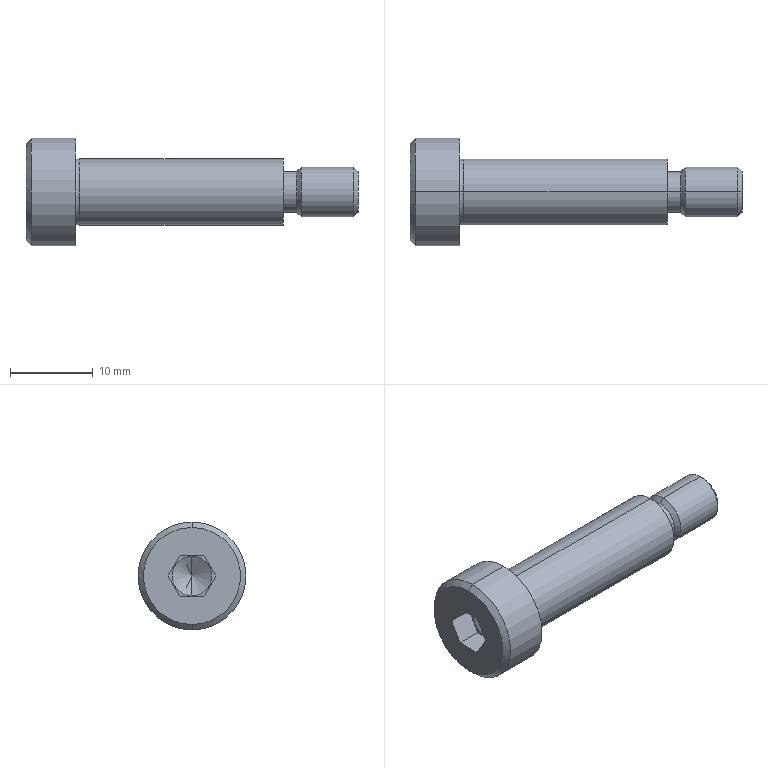Part | STEP file | MSB8-25 | 1 solid | 29 faces | box 40 x 13 x 13 mm | volume 2205 mm3 | plane 11 | cylinder 8 | cone 8 | spline 2 | commonest cylinder face diameters 4.917 x2 6 x2 8 x2 13 x2
STEP:
#1=CARTESIAN_POINT('',(0.48,0.,-4.));
#2=VERTEX_POINT('',#1);
#3=CARTESIAN_POINT('',(0.48,0.,4.));
#4=VERTEX_POINT('',#3);
#5=CARTESIAN_POINT('',(0.48,0.,0.));
#6=DIRECTION('',(1.,0.,0.));
#7=DIRECTION('',(0.,0.,-1.));
#8=AXIS2_PLACEMENT_3D('',#5,#6,#7);
#9=CIRCLE('',#8,4.);
#10=EDGE_CURVE('',#2,#4,#9,.T.);
#11=ORIENTED_EDGE('',*,*,#10,.F.);
#12=CARTESIAN_POINT('',(0.,0.,-4.));
#13=VERTEX_POINT('',#12);
#14=CARTESIAN_POINT('',(0.24,0.,-4.387));
#15=DIRECTION('',(0.,-1.,0.));
#16=DIRECTION('',(0.,0.,-1.));
#17=AXIS2_PLACEMENT_3D('',#14,#15,#16);
#18=CIRCLE('',#17,0.455);
#19=EDGE_CURVE('',#2,#13,#18,.T.);
#20=ORIENTED_EDGE('',*,*,#19,.T.);
#21=CARTESIAN_POINT('',(0.,0.,4.));
#22=VERTEX_POINT('',#21);
#23=CARTESIAN_POINT('',(0.,0.,0.));
#24=DIRECTION('',(-1.,0.,0.));
#25=DIRECTION('',(0.,0.,1.));
#26=AXIS2_PLACEMENT_3D('',#23,#24,#25);
#27=CIRCLE('',#26,4.);
#28=EDGE_CURVE('',#22,#13,#27,.T.);
#29=ORIENTED_EDGE('',*,*,#28,.F.);
#30=CARTESIAN_POINT('',(0.24,0.,4.387));
#31=DIRECTION('',(0.,1.,0.));
#32=DIRECTION('',(0.,0.,1.));
#33=AXIS2_PLACEMENT_3D('',#30,#31,#32);
#34=CIRCLE('',#33,0.455);
#35=EDGE_CURVE('',#4,#22,#34,.T.);
#36=ORIENTED_EDGE('',*,*,#35,.F.);
#37=EDGE_LOOP('',(#11,#20,#29,#36));
#38=FACE_OUTER_BOUND('',#37,.T.);
#39=CARTESIAN_POINT('',(0.48,0.,4.));
#40=CARTESIAN_POINT('',(0.48,8.,4.));
#41=CARTESIAN_POINT('',(0.48,8.,-4.));
#42=CARTESIAN_POINT('',(0.48,0.,-4.));
#43=CARTESIAN_POINT('',(0.3289,0.,3.906));
#44=CARTESIAN_POINT('',(0.3289,7.812,3.906));
#45=CARTESIAN_POINT('',(0.3289,7.812,-3.906));
#46=CARTESIAN_POINT('',(0.3289,0.,-3.906));
#47=CARTESIAN_POINT('',(0.1511,0.,3.906));
#48=CARTESIAN_POINT('',(0.1511,7.812,3.906));
#49=CARTESIAN_POINT('',(0.1511,7.812,-3.906));
#50=CARTESIAN_POINT('',(0.1511,0.,-3.906));
#51=CARTESIAN_POINT('',(0.,0.,4.));
#52=CARTESIAN_POINT('',(0.,8.,4.));
#53=CARTESIAN_POINT('',(0.,8.,-4.));
#54=CARTESIAN_POINT('',(0.,0.,-4.));
#55=(BOUNDED_SURFACE()B_SPLINE_SURFACE(3,3,((#39,#40,#41,#42),(#43,#44,#45,#46),(#47,#48,#49,#50),(#51,#52,#53,#54)),.UNSPECIFIED.,.F.,.F.,.F.)B_SPLINE_SURFACE_WITH_KNOTS((4,4),(4,4),(0.,1.),(0.,1.),.UNSPECIFIED.)GEOMETRIC_REPRESENTATION_ITEM()RATIONAL_B_SPLINE_SURFACE(((1.,0.3333,0.3333,1.),(0.8997,0.2999,0.2999,0.8997),(0.8997,0.2999,0.2999,0.8997),(1.,0.3333,0.3333,1.)))REPRESENTATION_ITEM('')SURFACE());
#56=ADVANCED_FACE('',(#38),#55,.F.);
#57=ORIENTED_EDGE('',*,*,#10,.T.);
#58=CARTESIAN_POINT('',(25.,0.,4.));
#59=VERTEX_POINT('',#58);
#60=CARTESIAN_POINT('',(12.74,0.,4.));
#61=DIRECTION('',(1.,0.,0.));
#62=VECTOR('',#61,1000.);
#63=LINE('',#60,#62);
#64=EDGE_CURVE('',#4,#59,#63,.T.);
#65=ORIENTED_EDGE('',*,*,#64,.T.);
#66=CARTESIAN_POINT('',(25.,0.,-4.));
#67=VERTEX_POINT('',#66);
#68=CARTESIAN_POINT('',(25.,0.,0.));
#69=DIRECTION('',(-1.,0.,0.));
#70=DIRECTION('',(0.,0.,-1.));
#71=AXIS2_PLACEMENT_3D('',#68,#69,#70);
#72=CIRCLE('',#71,4.);
#73=EDGE_CURVE('',#59,#67,#72,.T.);
#74=ORIENTED_EDGE('',*,*,#73,.T.);
#75=CARTESIAN_POINT('',(12.74,0.,-4.));
#76=DIRECTION('',(1.,0.,0.));
#77=VECTOR('',#76,1000.);
#78=LINE('',#75,#77);
#79=EDGE_CURVE('',#2,#67,#78,.T.);
#80=ORIENTED_EDGE('',*,*,#79,.F.);
#81=EDGE_LOOP('',(#57,#65,#74,#80));
#82=FACE_OUTER_BOUND('',#81,.T.);
#83=CARTESIAN_POINT('',(12.74,0.,0.));
#84=DIRECTION('',(1.,0.,0.));
#85=DIRECTION('',(0.,0.,-1.));
#86=AXIS2_PLACEMENT_3D('',#83,#84,#85);
#87=CYLINDRICAL_SURFACE('',#86,4.);
#88=ADVANCED_FACE('',(#82),#87,.T.);
#89=CARTESIAN_POINT('',(25.,0.,2.459));
#90=VERTEX_POINT('',#89);
#91=CARTESIAN_POINT('',(25.,0.,-2.459));
#92=VERTEX_POINT('',#91);
#93=CARTESIAN_POINT('',(25.,0.,0.));
#94=DIRECTION('',(-1.,0.,0.));
#95=DIRECTION('',(0.,0.,-1.));
#96=AXIS2_PLACEMENT_3D('',#93,#94,#95);
#97=CIRCLE('',#96,2.459);
#98=EDGE_CURVE('',#90,#92,#97,.T.);
#99=ORIENTED_EDGE('',*,*,#98,.F.);
#100=CARTESIAN_POINT('',(26.617,0.,2.459));
#101=VERTEX_POINT('',#100);
#102=CARTESIAN_POINT('',(25.809,0.,2.459));
#103=DIRECTION('',(1.,0.,0.));
#104=VECTOR('',#103,1000.);
#105=LINE('',#102,#104);
#106=EDGE_CURVE('',#90,#101,#105,.T.);
#107=ORIENTED_EDGE('',*,*,#106,.T.);
#108=CARTESIAN_POINT('',(26.617,0.,-2.459));
#109=VERTEX_POINT('',#108);
#110=CARTESIAN_POINT('',(26.617,0.,0.));
#111=DIRECTION('',(-1.,0.,0.));
#112=DIRECTION('',(0.,0.,-1.));
#113=AXIS2_PLACEMENT_3D('',#110,#111,#112);
#114=CIRCLE('',#113,2.459);
#115=EDGE_CURVE('',#101,#109,#114,.T.);
#116=ORIENTED_EDGE('',*,*,#115,.T.);
#117=CARTESIAN_POINT('',(25.809,0.,-2.459));
#118=DIRECTION('',(1.,0.,0.));
#119=VECTOR('',#118,1000.);
#120=LINE('',#117,#119);
#121=EDGE_CURVE('',#92,#109,#120,.T.);
#122=ORIENTED_EDGE('',*,*,#121,.F.);
#123=EDGE_LOOP('',(#99,#107,#116,#122));
#124=FACE_OUTER_BOUND('',#123,.T.);
#125=CARTESIAN_POINT('',(25.809,0.,0.));
#126=DIRECTION('',(1.,0.,0.));
#127=DIRECTION('',(0.,0.,-1.));
#128=AXIS2_PLACEMENT_3D('',#125,#126,#127);
#129=CYLINDRICAL_SURFACE('',#128,2.459);
#130=ADVANCED_FACE('',(#124),#129,.T.);
#131=ORIENTED_EDGE('',*,*,#115,.F.);
#132=CARTESIAN_POINT('',(27.158,0.,3.));
#133=VERTEX_POINT('',#132);
#134=CARTESIAN_POINT('',(27.158,0.,3.));
#135=DIRECTION('',(0.7071,0.,0.7071));
#136=VECTOR('',#135,1000.);
#137=LINE('',#134,#136);
#138=EDGE_CURVE('',#101,#133,#137,.T.);
#139=ORIENTED_EDGE('',*,*,#138,.T.);
#140=CARTESIAN_POINT('',(27.158,0.,-3.));
#141=VERTEX_POINT('',#140);
#142=CARTESIAN_POINT('',(27.158,0.,0.));
#143=DIRECTION('',(-1.,0.,0.));
#144=DIRECTION('',(0.,1.,0.));
#145=AXIS2_PLACEMENT_3D('',#142,#143,#144);
#146=CIRCLE('',#145,3.);
#147=EDGE_CURVE('',#133,#141,#146,.T.);
#148=ORIENTED_EDGE('',*,*,#147,.T.);
#149=CARTESIAN_POINT('',(27.158,0.,-3.));
#150=DIRECTION('',(0.7071,0.,-0.7071));
#151=VECTOR('',#150,1000.);
#152=LINE('',#149,#151);
#153=EDGE_CURVE('',#109,#141,#152,.T.);
#154=ORIENTED_EDGE('',*,*,#153,.F.);
#155=EDGE_LOOP('',(#131,#139,#148,#154));
#156=FACE_OUTER_BOUND('',#155,.T.);
#157=CARTESIAN_POINT('',(27.158,0.,0.));
#158=DIRECTION('',(1.,0.,0.));
#159=DIRECTION('',(0.,0.,-1.));
#160=AXIS2_PLACEMENT_3D('',#157,#158,#159);
#161=CONICAL_SURFACE('',#160,3.,0.7854);
#162=ADVANCED_FACE('',(#156),#161,.T.);
#163=CARTESIAN_POINT('',(-5.35,0.,-6.5));
#164=VERTEX_POINT('',#163);
#165=CARTESIAN_POINT('',(-5.35,0.,6.5));
#166=VERTEX_POINT('',#165);
#167=CARTESIAN_POINT('',(-5.35,0.,0.));
#168=DIRECTION('',(1.,0.,0.));
#169=DIRECTION('',(0.,0.,-1.));
#170=AXIS2_PLACEMENT_3D('',#167,#168,#169);
#171=CIRCLE('',#170,6.5);
#172=EDGE_CURVE('',#164,#166,#171,.T.);
#173=ORIENTED_EDGE('',*,*,#172,.T.);
#174=CARTESIAN_POINT('',(0.,0.,6.5));
#175=VERTEX_POINT('',#174);
#176=CARTESIAN_POINT('',(-2.675,0.,6.5));
#177=DIRECTION('',(1.,0.,0.));
#178=VECTOR('',#177,1000.);
#179=LINE('',#176,#178);
#180=EDGE_CURVE('',#166,#175,#179,.T.);
#181=ORIENTED_EDGE('',*,*,#180,.T.);
#182=CARTESIAN_POINT('',(0.,0.,-6.5));
#183=VERTEX_POINT('',#182);
#184=CARTESIAN_POINT('',(0.,0.,0.));
#185=DIRECTION('',(1.,0.,0.));
#186=DIRECTION('',(0.,0.,-1.));
#187=AXIS2_PLACEMENT_3D('',#184,#185,#186);
#188=CIRCLE('',#187,6.5);
#189=EDGE_CURVE('',#183,#175,#188,.T.);
#190=ORIENTED_EDGE('',*,*,#189,.F.);
#191=CARTESIAN_POINT('',(-2.675,0.,-6.5));
#192=DIRECTION('',(1.,0.,0.));
#193=VECTOR('',#192,1000.);
#194=LINE('',#191,#193);
#195=EDGE_CURVE('',#164,#183,#194,.T.);
#196=ORIENTED_EDGE('',*,*,#195,.F.);
#197=EDGE_LOOP('',(#173,#181,#190,#196));
#198=FACE_OUTER_BOUND('',#197,.T.);
#199=CARTESIAN_POINT('',(-2.675,0.,0.));
#200=DIRECTION('',(1.,0.,0.));
#201=DIRECTION('',(0.,0.,-1.));
#202=AXIS2_PLACEMENT_3D('',#199,#200,#201);
#203=CYLINDRICAL_SURFACE('',#202,6.5);
#204=ADVANCED_FACE('',(#198),#203,.T.);
#205=ORIENTED_EDGE('',*,*,#147,.F.);
#206=CARTESIAN_POINT('',(33.459,0.,3.));
#207=VERTEX_POINT('',#206);
#208=CARTESIAN_POINT('',(30.308,0.,3.));
#209=DIRECTION('',(1.,0.,0.));
#210=VECTOR('',#209,1000.);
#211=LINE('',#208,#210);
#212=EDGE_CURVE('',#133,#207,#211,.T.);
#213=ORIENTED_EDGE('',*,*,#212,.T.);
#214=CARTESIAN_POINT('',(33.459,0.,-3.));
#215=VERTEX_POINT('',#214);
#216=CARTESIAN_POINT('',(33.459,0.,0.));
#217=DIRECTION('',(-1.,0.,0.));
#218=DIRECTION('',(0.,0.,-1.));
#219=AXIS2_PLACEMENT_3D('',#216,#217,#218);
#220=CIRCLE('',#219,3.);
#221=EDGE_CURVE('',#207,#215,#220,.T.);
#222=ORIENTED_EDGE('',*,*,#221,.T.);
#223=CARTESIAN_POINT('',(30.308,0.,-3.));
#224=DIRECTION('',(1.,0.,0.));
#225=VECTOR('',#224,1000.);
#226=LINE('',#223,#225);
#227=EDGE_CURVE('',#141,#215,#226,.T.);
#228=ORIENTED_EDGE('',*,*,#227,.F.);
#229=EDGE_LOOP('',(#205,#213,#222,#228));
#230=FACE_OUTER_BOUND('',#229,.T.);
#231=CARTESIAN_POINT('',(30.308,0.,0.));
#232=DIRECTION('',(1.,0.,0.));
#233=DIRECTION('',(0.,0.,-1.));
#234=AXIS2_PLACEMENT_3D('',#231,#232,#233);
#235=CYLINDRICAL_SURFACE('',#234,3.);
#236=ADVANCED_FACE('',(#230),#235,.T.);
#237=CARTESIAN_POINT('',(-6.,0.,-5.85));
#238=VERTEX_POINT('',#237);
#239=CARTESIAN_POINT('',(-6.,0.,5.85));
#240=VERTEX_POINT('',#239);
#241=CARTESIAN_POINT('',(-6.,0.,0.));
#242=DIRECTION('',(1.,0.,0.));
#243=DIRECTION('',(0.,0.,-1.));
#244=AXIS2_PLACEMENT_3D('',#241,#242,#243);
#245=CIRCLE('',#244,5.85);
#246=EDGE_CURVE('',#238,#240,#245,.T.);
#247=ORIENTED_EDGE('',*,*,#246,.T.);
#248=CARTESIAN_POINT('',(-5.35,0.,6.5));
#249=DIRECTION('',(0.7071,0.,0.7071));
#250=VECTOR('',#249,1000.);
#251=LINE('',#248,#250);
#252=EDGE_CURVE('',#240,#166,#251,.T.);
#253=ORIENTED_EDGE('',*,*,#252,.T.);
#254=ORIENTED_EDGE('',*,*,#172,.F.);
#255=CARTESIAN_POINT('',(-5.35,0.,-6.5));
#256=DIRECTION('',(0.7071,0.,-0.7071));
#257=VECTOR('',#256,1000.);
#258=LINE('',#255,#257);
#259=EDGE_CURVE('',#238,#164,#258,.T.);
#260=ORIENTED_EDGE('',*,*,#259,.F.);
#261=EDGE_LOOP('',(#247,#253,#254,#260));
#262=FACE_OUTER_BOUND('',#261,.T.);
#263=CARTESIAN_POINT('',(-5.35,0.,0.));
#264=DIRECTION('',(1.,0.,0.));
#265=DIRECTION('',(0.,0.,-1.));
#266=AXIS2_PLACEMENT_3D('',#263,#264,#265);
#267=CONICAL_SURFACE('',#266,6.5,0.7854);
#268=ADVANCED_FACE('',(#262),#267,.T.);
#269=CARTESIAN_POINT('',(34.,0.,2.459));
#270=VERTEX_POINT('',#269);
#271=CARTESIAN_POINT('',(34.,0.,-2.459));
#272=VERTEX_POINT('',#271);
#273=CARTESIAN_POINT('',(34.,0.,0.));
#274=DIRECTION('',(-1.,0.,0.));
#275=DIRECTION('',(0.,0.,1.));
#276=AXIS2_PLACEMENT_3D('',#273,#274,#275);
#277=CIRCLE('',#276,2.459);
#278=EDGE_CURVE('',#270,#272,#277,.T.);
#279=ORIENTED_EDGE('',*,*,#278,.T.);
#280=CARTESIAN_POINT('',(33.459,0.,-3.));
#281=DIRECTION('',(-0.7071,0.,-0.7071));
#282=VECTOR('',#281,1000.);
#283=LINE('',#280,#282);
#284=EDGE_CURVE('',#272,#215,#283,.T.);
#285=ORIENTED_EDGE('',*,*,#284,.T.);
#286=ORIENTED_EDGE('',*,*,#221,.F.);
#287=CARTESIAN_POINT('',(33.459,0.,3.));
#288=DIRECTION('',(-0.7071,0.,0.7071));
#289=VECTOR('',#288,1000.);
#290=LINE('',#287,#289);
#291=EDGE_CURVE('',#270,#207,#290,.T.);
#292=ORIENTED_EDGE('',*,*,#291,.F.);
#293=EDGE_LOOP('',(#279,#285,#286,#292));
#294=FACE_OUTER_BOUND('',#293,.T.);
#295=CARTESIAN_POINT('',(33.459,0.,0.));
#296=DIRECTION('',(-1.,0.,0.));
#297=DIRECTION('',(0.,0.,1.));
#298=AXIS2_PLACEMENT_3D('',#295,#296,#297);
#299=CONICAL_SURFACE('',#298,3.,0.7854);
#300=ADVANCED_FACE('',(#294),#299,.T.);
#301=CARTESIAN_POINT('',(-1.614,0.,0.));
#302=VERTEX_POINT('',#301);
#303=CARTESIAN_POINT('',(-3.,0.,2.4));
#304=VERTEX_POINT('',#303);
#305=CARTESIAN_POINT('',(-3.,0.,2.4));
#306=DIRECTION('',(-0.5,0.,0.866));
#307=VECTOR('',#306,1000.);
#308=LINE('',#305,#307);
#309=EDGE_CURVE('',#302,#304,#308,.T.);
#310=ORIENTED_EDGE('',*,*,#309,.F.);
#311=CARTESIAN_POINT('',(-3.,0.,-2.4));
#312=VERTEX_POINT('',#311);
#313=CARTESIAN_POINT('',(-3.,0.,-2.4));
#314=DIRECTION('',(-0.5,0.,-0.866));
#315=VECTOR('',#314,1000.);
#316=LINE('',#313,#315);
#317=EDGE_CURVE('',#302,#312,#316,.T.);
#318=ORIENTED_EDGE('',*,*,#317,.T.);
#319=CARTESIAN_POINT('',(-3.,0.,0.));
#320=DIRECTION('',(-1.,0.,0.));
#321=DIRECTION('',(0.,0.,1.));
#322=AXIS2_PLACEMENT_3D('',#319,#320,#321);
#323=CIRCLE('',#322,2.4);
#324=EDGE_CURVE('',#312,#304,#323,.T.);
#325=ORIENTED_EDGE('',*,*,#324,.T.);
#326=EDGE_LOOP('',(#310,#318,#325));
#327=FACE_OUTER_BOUND('',#326,.T.);
#328=CARTESIAN_POINT('',(-3.,0.,0.));
#329=DIRECTION('',(-1.,0.,0.));
#330=DIRECTION('',(0.,0.,1.));
#331=AXIS2_PLACEMENT_3D('',#328,#329,#330);
#332=CONICAL_SURFACE('',#331,2.4,1.047);
#333=ADVANCED_FACE('',(#327),#332,.F.);
#334=ORIENTED_EDGE('',*,*,#64,.F.);
#335=CARTESIAN_POINT('',(0.48,0.,0.));
#336=DIRECTION('',(1.,0.,0.));
#337=DIRECTION('',(0.,0.,-1.));
#338=AXIS2_PLACEMENT_3D('',#335,#336,#337);
#339=CIRCLE('',#338,4.);
#340=EDGE_CURVE('',#4,#2,#339,.T.);
#341=ORIENTED_EDGE('',*,*,#340,.T.);
#342=ORIENTED_EDGE('',*,*,#79,.T.);
#343=CARTESIAN_POINT('',(25.,0.,0.));
#344=DIRECTION('',(-1.,0.,0.));
#345=DIRECTION('',(0.,0.,-1.));
#346=AXIS2_PLACEMENT_3D('',#343,#344,#345);
#347=CIRCLE('',#346,4.);
#348=EDGE_CURVE('',#67,#59,#347,.T.);
#349=ORIENTED_EDGE('',*,*,#348,.T.);
#350=EDGE_LOOP('',(#334,#341,#342,#349));
#351=FACE_OUTER_BOUND('',#350,.T.);
#352=CARTESIAN_POINT('',(12.74,0.,0.));
#353=DIRECTION('',(1.,0.,0.));
#354=DIRECTION('',(0.,0.,-1.));
#355=AXIS2_PLACEMENT_3D('',#352,#353,#354);
#356=CYLINDRICAL_SURFACE('',#355,4.);
#357=ADVANCED_FACE('',(#351),#356,.T.);
#358=ORIENTED_EDGE('',*,*,#19,.F.);
#359=ORIENTED_EDGE('',*,*,#340,.F.);
#360=ORIENTED_EDGE('',*,*,#35,.T.);
#361=CARTESIAN_POINT('',(0.,0.,0.));
#362=DIRECTION('',(-1.,0.,0.));
#363=DIRECTION('',(0.,0.,1.));
#364=AXIS2_PLACEMENT_3D('',#361,#362,#363);
#365=CIRCLE('',#364,4.);
#366=EDGE_CURVE('',#13,#22,#365,.T.);
#367=ORIENTED_EDGE('',*,*,#366,.F.);
#368=EDGE_LOOP('',(#358,#359,#360,#367));
#369=FACE_OUTER_BOUND('',#368,.T.);
#370=CARTESIAN_POINT('',(0.48,0.,-4.));
#371=CARTESIAN_POINT('',(0.48,-8.,-4.));
#372=CARTESIAN_POINT('',(0.48,-8.,4.));
#373=CARTESIAN_POINT('',(0.48,0.,4.));
#374=CARTESIAN_POINT('',(0.3289,0.,-3.906));
#375=CARTESIAN_POINT('',(0.3289,-7.812,-3.906));
#376=CARTESIAN_POINT('',(0.3289,-7.812,3.906));
#377=CARTESIAN_POINT('',(0.3289,0.,3.906));
#378=CARTESIAN_POINT('',(0.1511,0.,-3.906));
#379=CARTESIAN_POINT('',(0.1511,-7.812,-3.906));
#380=CARTESIAN_POINT('',(0.1511,-7.812,3.906));
#381=CARTESIAN_POINT('',(0.1511,0.,3.906));
#382=CARTESIAN_POINT('',(0.,0.,-4.));
#383=CARTESIAN_POINT('',(0.,-8.,-4.));
#384=CARTESIAN_POINT('',(0.,-8.,4.));
#385=CARTESIAN_POINT('',(0.,0.,4.));
#386=(BOUNDED_SURFACE()B_SPLINE_SURFACE(3,3,((#370,#371,#372,#373),(#374,#375,#376,#377),(#378,#379,#380,#381),(#382,#383,#384,#385)),.UNSPECIFIED.,.F.,.F.,.F.)B_SPLINE_SURFACE_WITH_KNOTS((4,4),(4,4),(0.,1.),(0.,1.),.UNSPECIFIED.)GEOMETRIC_REPRESENTATION_ITEM()RATIONAL_B_SPLINE_SURFACE(((1.,0.3333,0.3333,1.),(0.8997,0.2999,0.2999,0.8997),(0.8997,0.2999,0.2999,0.8997),(1.,0.3333,0.3333,1.)))REPRESENTATION_ITEM('')SURFACE());
#387=ADVANCED_FACE('',(#369),#386,.F.);
#388=CARTESIAN_POINT('',(25.,0.,0.));
#389=DIRECTION('',(-1.,0.,0.));
#390=DIRECTION('',(0.,0.,-1.));
#391=AXIS2_PLACEMENT_3D('',#388,#389,#390);
#392=CIRCLE('',#391,2.459);
#393=EDGE_CURVE('',#92,#90,#392,.T.);
#394=ORIENTED_EDGE('',*,*,#393,.T.);
#395=ORIENTED_EDGE('',*,*,#98,.T.);
#396=EDGE_LOOP('',(#394,#395));
#397=FACE_BOUND('',#396,.T.);
#398=ORIENTED_EDGE('',*,*,#348,.F.);
#399=ORIENTED_EDGE('',*,*,#73,.F.);
#400=EDGE_LOOP('',(#398,#399));
#401=FACE_OUTER_BOUND('',#400,.T.);
#402=CARTESIAN_POINT('',(25.,3.229,0.));
#403=DIRECTION('',(1.,0.,0.));
#404=DIRECTION('',(0.,0.,-1.));
#405=AXIS2_PLACEMENT_3D('',#402,#403,#404);
#406=PLANE('',#405);
#407=ADVANCED_FACE('',(#397,#401),#406,.T.);
#408=ORIENTED_EDGE('',*,*,#106,.F.);
#409=ORIENTED_EDGE('',*,*,#393,.F.);
#410=ORIENTED_EDGE('',*,*,#121,.T.);
#411=CARTESIAN_POINT('',(26.617,0.,0.));
#412=DIRECTION('',(-1.,0.,0.));
#413=DIRECTION('',(0.,0.,-1.));
#414=AXIS2_PLACEMENT_3D('',#411,#412,#413);
#415=CIRCLE('',#414,2.459);
#416=EDGE_CURVE('',#109,#101,#415,.T.);
#417=ORIENTED_EDGE('',*,*,#416,.T.);
#418=EDGE_LOOP('',(#408,#409,#410,#417));
#419=FACE_OUTER_BOUND('',#418,.T.);
#420=CARTESIAN_POINT('',(25.809,0.,0.));
#421=DIRECTION('',(1.,0.,0.));
#422=DIRECTION('',(0.,0.,-1.));
#423=AXIS2_PLACEMENT_3D('',#420,#421,#422);
#424=CYLINDRICAL_SURFACE('',#423,2.459);
#425=ADVANCED_FACE('',(#419),#424,.T.);
#426=ORIENTED_EDGE('',*,*,#28,.T.);
#427=ORIENTED_EDGE('',*,*,#366,.T.);
#428=EDGE_LOOP('',(#426,#427));
#429=FACE_BOUND('',#428,.T.);
#430=ORIENTED_EDGE('',*,*,#189,.T.);
#431=CARTESIAN_POINT('',(0.,0.,0.));
#432=DIRECTION('',(1.,0.,0.));
#433=DIRECTION('',(0.,0.,-1.));
#434=AXIS2_PLACEMENT_3D('',#431,#432,#433);
#435=CIRCLE('',#434,6.5);
#436=EDGE_CURVE('',#175,#183,#435,.T.);
#437=ORIENTED_EDGE('',*,*,#436,.T.);
#438=EDGE_LOOP('',(#430,#437));
#439=FACE_OUTER_BOUND('',#438,.T.);
#440=CARTESIAN_POINT('',(0.,5.25,0.));
#441=DIRECTION('',(1.,0.,0.));
#442=DIRECTION('',(0.,0.,-1.));
#443=AXIS2_PLACEMENT_3D('',#440,#441,#442);
#444=PLANE('',#443);
#445=ADVANCED_FACE('',(#429,#439),#444,.T.);
#446=ORIENTED_EDGE('',*,*,#138,.F.);
#447=ORIENTED_EDGE('',*,*,#416,.F.);
#448=ORIENTED_EDGE('',*,*,#153,.T.);
#449=CARTESIAN_POINT('',(27.158,0.,0.));
#450=DIRECTION('',(-1.,0.,0.));
#451=DIRECTION('',(0.,1.,0.));
#452=AXIS2_PLACEMENT_3D('',#449,#450,#451);
#453=CIRCLE('',#452,3.);
#454=EDGE_CURVE('',#141,#133,#453,.T.);
#455=ORIENTED_EDGE('',*,*,#454,.T.);
#456=EDGE_LOOP('',(#446,#447,#448,#455));
#457=FACE_OUTER_BOUND('',#456,.T.);
#458=CARTESIAN_POINT('',(27.158,0.,0.));
#459=DIRECTION('',(1.,0.,0.));
#460=DIRECTION('',(0.,0.,-1.));
#461=AXIS2_PLACEMENT_3D('',#458,#459,#460);
#462=CONICAL_SURFACE('',#461,3.,0.7854);
#463=ADVANCED_FACE('',(#457),#462,.T.);
#464=ORIENTED_EDGE('',*,*,#180,.F.);
#465=CARTESIAN_POINT('',(-5.35,0.,0.));
#466=DIRECTION('',(1.,0.,0.));
#467=DIRECTION('',(0.,0.,-1.));
#468=AXIS2_PLACEMENT_3D('',#465,#466,#467);
#469=CIRCLE('',#468,6.5);
#470=EDGE_CURVE('',#166,#164,#469,.T.);
#471=ORIENTED_EDGE('',*,*,#470,.T.);
#472=ORIENTED_EDGE('',*,*,#195,.T.);
#473=ORIENTED_EDGE('',*,*,#436,.F.);
#474=EDGE_LOOP('',(#464,#471,#472,#473));
#475=FACE_OUTER_BOUND('',#474,.T.);
#476=CARTESIAN_POINT('',(-2.675,0.,0.));
#477=DIRECTION('',(1.,0.,0.));
#478=DIRECTION('',(0.,0.,-1.));
#479=AXIS2_PLACEMENT_3D('',#476,#477,#478);
#480=CYLINDRICAL_SURFACE('',#479,6.5);
#481=ADVANCED_FACE('',(#475),#480,.T.);
#482=ORIENTED_EDGE('',*,*,#212,.F.);
#483=ORIENTED_EDGE('',*,*,#454,.F.);
#484=ORIENTED_EDGE('',*,*,#227,.T.);
#485=CARTESIAN_POINT('',(33.459,0.,0.));
#486=DIRECTION('',(-1.,0.,0.));
#487=DIRECTION('',(0.,0.,-1.));
#488=AXIS2_PLACEMENT_3D('',#485,#486,#487);
#489=CIRCLE('',#488,3.);
#490=EDGE_CURVE('',#215,#207,#489,.T.);
#491=ORIENTED_EDGE('',*,*,#490,.T.);
#492=EDGE_LOOP('',(#482,#483,#484,#491));
#493=FACE_OUTER_BOUND('',#492,.T.);
#494=CARTESIAN_POINT('',(30.308,0.,0.));
#495=DIRECTION('',(1.,0.,0.));
#496=DIRECTION('',(0.,0.,-1.));
#497=AXIS2_PLACEMENT_3D('',#494,#495,#496);
#498=CYLINDRICAL_SURFACE('',#497,3.);
#499=ADVANCED_FACE('',(#493),#498,.T.);
#500=ORIENTED_EDGE('',*,*,#252,.F.);
#501=CARTESIAN_POINT('',(-6.,0.,0.));
#502=DIRECTION('',(1.,0.,0.));
#503=DIRECTION('',(0.,0.,-1.));
#504=AXIS2_PLACEMENT_3D('',#501,#502,#503);
#505=CIRCLE('',#504,5.85);
#506=EDGE_CURVE('',#240,#238,#505,.T.);
#507=ORIENTED_EDGE('',*,*,#506,.T.);
#508=ORIENTED_EDGE('',*,*,#259,.T.);
#509=ORIENTED_EDGE('',*,*,#470,.F.);
#510=EDGE_LOOP('',(#500,#507,#508,#509));
#511=FACE_OUTER_BOUND('',#510,.T.);
#512=CARTESIAN_POINT('',(-5.35,0.,0.));
#513=DIRECTION('',(1.,0.,0.));
#514=DIRECTION('',(0.,0.,-1.));
#515=AXIS2_PLACEMENT_3D('',#512,#513,#514);
#516=CONICAL_SURFACE('',#515,6.5,0.7854);
#517=ADVANCED_FACE('',(#511),#516,.T.);
#518=ORIENTED_EDGE('',*,*,#284,.F.);
#519=CARTESIAN_POINT('',(34.,0.,0.));
#520=DIRECTION('',(-1.,0.,0.));
#521=DIRECTION('',(0.,0.,1.));
#522=AXIS2_PLACEMENT_3D('',#519,#520,#521);
#523=CIRCLE('',#522,2.459);
#524=EDGE_CURVE('',#272,#270,#523,.T.);
#525=ORIENTED_EDGE('',*,*,#524,.T.);
#526=ORIENTED_EDGE('',*,*,#291,.T.);
#527=ORIENTED_EDGE('',*,*,#490,.F.);
#528=EDGE_LOOP('',(#518,#525,#526,#527));
#529=FACE_OUTER_BOUND('',#528,.T.);
#530=CARTESIAN_POINT('',(33.459,0.,0.));
#531=DIRECTION('',(-1.,0.,0.));
#532=DIRECTION('',(0.,0.,1.));
#533=AXIS2_PLACEMENT_3D('',#530,#531,#532);
#534=CONICAL_SURFACE('',#533,3.,0.7854);
#535=ADVANCED_FACE('',(#529),#534,.T.);
#536=ORIENTED_EDGE('',*,*,#246,.F.);
#537=ORIENTED_EDGE('',*,*,#506,.F.);
#538=EDGE_LOOP('',(#536,#537));
#539=FACE_OUTER_BOUND('',#538,.T.);
#540=CARTESIAN_POINT('',(-6.,-1.443,-2.5));
#541=VERTEX_POINT('',#540);
#542=CARTESIAN_POINT('',(-6.,1.443,-2.5));
#543=VERTEX_POINT('',#542);
#544=CARTESIAN_POINT('',(-6.,4.125,-2.5));
#545=DIRECTION('',(0.,1.,0.));
#546=VECTOR('',#545,1000.);
#547=LINE('',#544,#546);
#548=EDGE_CURVE('',#541,#543,#547,.T.);
#549=ORIENTED_EDGE('',*,*,#548,.T.);
#550=CARTESIAN_POINT('',(-6.,2.887,0.));
#551=VERTEX_POINT('',#550);
#552=CARTESIAN_POINT('',(-6.,1.443,-2.5));
#553=DIRECTION('',(0.,0.5,0.866));
#554=VECTOR('',#553,1000.);
#555=LINE('',#552,#554);
#556=EDGE_CURVE('',#543,#551,#555,.T.);
#557=ORIENTED_EDGE('',*,*,#556,.T.);
#558=CARTESIAN_POINT('',(-6.,1.443,2.5));
#559=VERTEX_POINT('',#558);
#560=CARTESIAN_POINT('',(-6.,2.887,0.));
#561=DIRECTION('',(0.,-0.5,0.866));
#562=VECTOR('',#561,1000.);
#563=LINE('',#560,#562);
#564=EDGE_CURVE('',#551,#559,#563,.T.);
#565=ORIENTED_EDGE('',*,*,#564,.T.);
#566=CARTESIAN_POINT('',(-6.,-1.443,2.5));
#567=VERTEX_POINT('',#566);
#568=CARTESIAN_POINT('',(-6.,4.125,2.5));
#569=DIRECTION('',(0.,-1.,0.));
#570=VECTOR('',#569,1000.);
#571=LINE('',#568,#570);
#572=EDGE_CURVE('',#559,#567,#571,.T.);
#573=ORIENTED_EDGE('',*,*,#572,.T.);
#574=CARTESIAN_POINT('',(-6.,-2.887,0.));
#575=VERTEX_POINT('',#574);
#576=CARTESIAN_POINT('',(-6.,-1.443,2.5));
#577=DIRECTION('',(0.,-0.5,-0.866));
#578=VECTOR('',#577,1000.);
#579=LINE('',#576,#578);
#580=EDGE_CURVE('',#567,#575,#579,.T.);
#581=ORIENTED_EDGE('',*,*,#580,.T.);
#582=CARTESIAN_POINT('',(-6.,-2.887,0.));
#583=DIRECTION('',(0.,0.5,-0.866));
#584=VECTOR('',#583,1000.);
#585=LINE('',#582,#584);
#586=EDGE_CURVE('',#575,#541,#585,.T.);
#587=ORIENTED_EDGE('',*,*,#586,.T.);
#588=EDGE_LOOP('',(#549,#557,#565,#573,#581,#587));
#589=FACE_BOUND('',#588,.T.);
#590=CARTESIAN_POINT('',(-6.,4.125,0.));
#591=DIRECTION('',(-1.,0.,0.));
#592=DIRECTION('',(0.,0.,1.));
#593=AXIS2_PLACEMENT_3D('',#590,#591,#592);
#594=PLANE('',#593);
#595=ADVANCED_FACE('',(#539,#589),#594,.T.);
#596=ORIENTED_EDGE('',*,*,#278,.F.);
#597=ORIENTED_EDGE('',*,*,#524,.F.);
#598=EDGE_LOOP('',(#596,#597));
#599=FACE_OUTER_BOUND('',#598,.T.);
#600=CARTESIAN_POINT('',(34.,1.229,0.));
#601=DIRECTION('',(1.,0.,0.));
#602=DIRECTION('',(0.,0.,-1.));
#603=AXIS2_PLACEMENT_3D('',#600,#601,#602);
#604=PLANE('',#603);
#605=ADVANCED_FACE('',(#599),#604,.T.);
#606=CARTESIAN_POINT('',(-3.,2.887,0.));
#607=VERTEX_POINT('',#606);
#608=CARTESIAN_POINT('',(-6.,2.887,0.));
#609=DIRECTION('',(1.,0.,0.));
#610=VECTOR('',#609,1000.);
#611=LINE('',#608,#610);
#612=EDGE_CURVE('',#551,#607,#611,.T.);
#613=ORIENTED_EDGE('',*,*,#612,.F.);
#614=ORIENTED_EDGE('',*,*,#556,.F.);
#615=CARTESIAN_POINT('',(-3.,1.443,-2.5));
#616=VERTEX_POINT('',#615);
#617=CARTESIAN_POINT('',(-6.,1.443,-2.5));
#618=DIRECTION('',(-1.,0.,0.));
#619=VECTOR('',#618,1000.);
#620=LINE('',#617,#619);
#621=EDGE_CURVE('',#616,#543,#620,.T.);
#622=ORIENTED_EDGE('',*,*,#621,.F.);
#623=CARTESIAN_POINT('',(-3.,2.887,0.));
#624=DIRECTION('',(0.,-0.5,-0.866));
#625=VECTOR('',#624,1000.);
#626=LINE('',#623,#625);
#627=EDGE_CURVE('',#607,#616,#626,.T.);
#628=ORIENTED_EDGE('',*,*,#627,.F.);
#629=EDGE_LOOP('',(#613,#614,#622,#628));
#630=FACE_OUTER_BOUND('',#629,.T.);
#631=CARTESIAN_POINT('',(-6.,2.887,0.));
#632=DIRECTION('',(0.,0.866,-0.5));
#633=DIRECTION('',(0.,0.5,0.866));
#634=AXIS2_PLACEMENT_3D('',#631,#632,#633);
#635=PLANE('',#634);
#636=ADVANCED_FACE('',(#630),#635,.F.);
#637=ORIENTED_EDGE('',*,*,#621,.T.);
#638=ORIENTED_EDGE('',*,*,#548,.F.);
#639=CARTESIAN_POINT('',(-3.,-1.443,-2.5));
#640=VERTEX_POINT('',#639);
#641=CARTESIAN_POINT('',(-6.,-1.443,-2.5));
#642=DIRECTION('',(-1.,0.,0.));
#643=VECTOR('',#642,1000.);
#644=LINE('',#641,#643);
#645=EDGE_CURVE('',#640,#541,#644,.T.);
#646=ORIENTED_EDGE('',*,*,#645,.F.);
#647=CARTESIAN_POINT('',(-3.,1.443,-2.5));
#648=DIRECTION('',(0.,-1.,0.));
#649=VECTOR('',#648,1000.);
#650=LINE('',#647,#649);
#651=EDGE_CURVE('',#616,#640,#650,.T.);
#652=ORIENTED_EDGE('',*,*,#651,.F.);
#653=EDGE_LOOP('',(#637,#638,#646,#652));
#654=FACE_OUTER_BOUND('',#653,.T.);
#655=CARTESIAN_POINT('',(-6.,1.443,-2.5));
#656=DIRECTION('',(0.,0.,-1.));
#657=DIRECTION('',(-1.,0.,0.));
#658=AXIS2_PLACEMENT_3D('',#655,#656,#657);
#659=PLANE('',#658);
#660=ADVANCED_FACE('',(#654),#659,.F.);
#661=ORIENTED_EDGE('',*,*,#645,.T.);
#662=ORIENTED_EDGE('',*,*,#586,.F.);
#663=CARTESIAN_POINT('',(-3.,-2.887,0.));
#664=VERTEX_POINT('',#663);
#665=CARTESIAN_POINT('',(-6.,-2.887,0.));
#666=DIRECTION('',(-1.,0.,0.));
#667=VECTOR('',#666,1000.);
#668=LINE('',#665,#667);
#669=EDGE_CURVE('',#664,#575,#668,.T.);
#670=ORIENTED_EDGE('',*,*,#669,.F.);
#671=CARTESIAN_POINT('',(-3.,-1.443,-2.5));
#672=DIRECTION('',(0.,-0.5,0.866));
#673=VECTOR('',#672,1000.);
#674=LINE('',#671,#673);
#675=EDGE_CURVE('',#640,#664,#674,.T.);
#676=ORIENTED_EDGE('',*,*,#675,.F.);
#677=EDGE_LOOP('',(#661,#662,#670,#676));
#678=FACE_OUTER_BOUND('',#677,.T.);
#679=CARTESIAN_POINT('',(-6.,-1.443,-2.5));
#680=DIRECTION('',(0.,-0.866,-0.5));
#681=DIRECTION('',(0.,0.5,-0.866));
#682=AXIS2_PLACEMENT_3D('',#679,#680,#681);
#683=PLANE('',#682);
#684=ADVANCED_FACE('',(#678),#683,.F.);
#685=ORIENTED_EDGE('',*,*,#669,.T.);
#686=ORIENTED_EDGE('',*,*,#580,.F.);
#687=CARTESIAN_POINT('',(-3.,-1.443,2.5));
#688=VERTEX_POINT('',#687);
#689=CARTESIAN_POINT('',(-6.,-1.443,2.5));
#690=DIRECTION('',(-1.,0.,0.));
#691=VECTOR('',#690,1000.);
#692=LINE('',#689,#691);
#693=EDGE_CURVE('',#688,#567,#692,.T.);
#694=ORIENTED_EDGE('',*,*,#693,.F.);
#695=CARTESIAN_POINT('',(-3.,-2.887,0.));
#696=DIRECTION('',(0.,0.5,0.866));
#697=VECTOR('',#696,1000.);
#698=LINE('',#695,#697);
#699=EDGE_CURVE('',#664,#688,#698,.T.);
#700=ORIENTED_EDGE('',*,*,#699,.F.);
#701=EDGE_LOOP('',(#685,#686,#694,#700));
#702=FACE_OUTER_BOUND('',#701,.T.);
#703=CARTESIAN_POINT('',(-6.,-2.887,0.));
#704=DIRECTION('',(0.,-0.866,0.5));
#705=DIRECTION('',(0.,-0.5,-0.866));
#706=AXIS2_PLACEMENT_3D('',#703,#704,#705);
#707=PLANE('',#706);
#708=ADVANCED_FACE('',(#702),#707,.F.);
#709=ORIENTED_EDGE('',*,*,#693,.T.);
#710=ORIENTED_EDGE('',*,*,#572,.F.);
#711=CARTESIAN_POINT('',(-3.,1.443,2.5));
#712=VERTEX_POINT('',#711);
#713=CARTESIAN_POINT('',(-6.,1.443,2.5));
#714=DIRECTION('',(-1.,0.,0.));
#715=VECTOR('',#714,1000.);
#716=LINE('',#713,#715);
#717=EDGE_CURVE('',#712,#559,#716,.T.);
#718=ORIENTED_EDGE('',*,*,#717,.F.);
#719=CARTESIAN_POINT('',(-3.,-1.443,2.5));
#720=DIRECTION('',(0.,1.,0.));
#721=VECTOR('',#720,1000.);
#722=LINE('',#719,#721);
#723=EDGE_CURVE('',#688,#712,#722,.T.);
#724=ORIENTED_EDGE('',*,*,#723,.F.);
#725=EDGE_LOOP('',(#709,#710,#718,#724));
#726=FACE_OUTER_BOUND('',#725,.T.);
#727=CARTESIAN_POINT('',(-6.,-1.443,2.5));
#728=DIRECTION('',(0.,0.,1.));
#729=DIRECTION('',(1.,0.,0.));
#730=AXIS2_PLACEMENT_3D('',#727,#728,#729);
#731=PLANE('',#730);
#732=ADVANCED_FACE('',(#726),#731,.F.);
#733=ORIENTED_EDGE('',*,*,#717,.T.);
#734=ORIENTED_EDGE('',*,*,#564,.F.);
#735=ORIENTED_EDGE('',*,*,#612,.T.);
#736=CARTESIAN_POINT('',(-3.,1.443,2.5));
#737=DIRECTION('',(0.,0.5,-0.866));
#738=VECTOR('',#737,1000.);
#739=LINE('',#736,#738);
#740=EDGE_CURVE('',#712,#607,#739,.T.);
#741=ORIENTED_EDGE('',*,*,#740,.F.);
#742=EDGE_LOOP('',(#733,#734,#735,#741));
#743=FACE_OUTER_BOUND('',#742,.T.);
#744=CARTESIAN_POINT('',(-6.,1.443,2.5));
#745=DIRECTION('',(0.,0.866,0.5));
#746=DIRECTION('',(0.,-0.5,0.866));
#747=AXIS2_PLACEMENT_3D('',#744,#745,#746);
#748=PLANE('',#747);
#749=ADVANCED_FACE('',(#743),#748,.F.);
#750=ORIENTED_EDGE('',*,*,#627,.T.);
#751=ORIENTED_EDGE('',*,*,#651,.T.);
#752=ORIENTED_EDGE('',*,*,#675,.T.);
#753=ORIENTED_EDGE('',*,*,#699,.T.);
#754=ORIENTED_EDGE('',*,*,#723,.T.);
#755=ORIENTED_EDGE('',*,*,#740,.T.);
#756=EDGE_LOOP('',(#750,#751,#752,#753,#754,#755));
#757=FACE_OUTER_BOUND('',#756,.T.);
#758=CARTESIAN_POINT('',(-3.,0.,0.));
#759=DIRECTION('',(-1.,0.,0.));
#760=DIRECTION('',(0.,0.,1.));
#761=AXIS2_PLACEMENT_3D('',#758,#759,#760);
#762=CIRCLE('',#761,2.4);
#763=EDGE_CURVE('',#304,#312,#762,.T.);
#764=ORIENTED_EDGE('',*,*,#763,.F.);
#765=ORIENTED_EDGE('',*,*,#324,.F.);
#766=EDGE_LOOP('',(#764,#765));
#767=FACE_BOUND('',#766,.T.);
#768=CARTESIAN_POINT('',(-3.,0.,0.));
#769=DIRECTION('',(1.,0.,0.));
#770=DIRECTION('',(0.,0.,-1.));
#771=AXIS2_PLACEMENT_3D('',#768,#769,#770);
#772=PLANE('',#771);
#773=ADVANCED_FACE('',(#757,#767),#772,.F.);
#774=ORIENTED_EDGE('',*,*,#317,.F.);
#775=ORIENTED_EDGE('',*,*,#309,.T.);
#776=ORIENTED_EDGE('',*,*,#763,.T.);
#777=EDGE_LOOP('',(#774,#775,#776));
#778=FACE_OUTER_BOUND('',#777,.T.);
#779=CARTESIAN_POINT('',(-3.,0.,0.));
#780=DIRECTION('',(-1.,0.,0.));
#781=DIRECTION('',(0.,0.,1.));
#782=AXIS2_PLACEMENT_3D('',#779,#780,#781);
#783=CONICAL_SURFACE('',#782,2.4,1.047);
#784=ADVANCED_FACE('',(#778),#783,.F.);
#785=CLOSED_SHELL('',(#56,#88,#130,#162,#204,#236,#268,#300,#333,#357,#387,#407,#425,#445,#463,#481,#499,#517,#535,#595,#605,#636,#660,#684,#708,#732,#749,#773,#784));
#786=MANIFOLD_SOLID_BREP('',#785);
#787=CARTESIAN_POINT('',(0.,0.,0.));
#788=DIRECTION('',(0.,0.,1.));
#789=DIRECTION('',(1.,0.,0.));
#790=AXIS2_PLACEMENT_3D('',#787,#788,#789);
#791=(LENGTH_UNIT()NAMED_UNIT(*)SI_UNIT(.MILLI.,.METRE.));
#792=UNCERTAINTY_MEASURE_WITH_UNIT(LENGTH_MEASURE(0.00001),#791,'','');
#793=(NAMED_UNIT(*)PLANE_ANGLE_UNIT()SI_UNIT($,.RADIAN.));
#794=(NAMED_UNIT(*)SI_UNIT($,.STERADIAN.)SOLID_ANGLE_UNIT());
#795=(GEOMETRIC_REPRESENTATION_CONTEXT(3)GLOBAL_UNCERTAINTY_ASSIGNED_CONTEXT((#792))GLOBAL_UNIT_ASSIGNED_CONTEXT((#791,#793,#794))REPRESENTATION_CONTEXT('',''));
#796=ADVANCED_BREP_SHAPE_REPRESENTATION('',(#786,#790),#795);